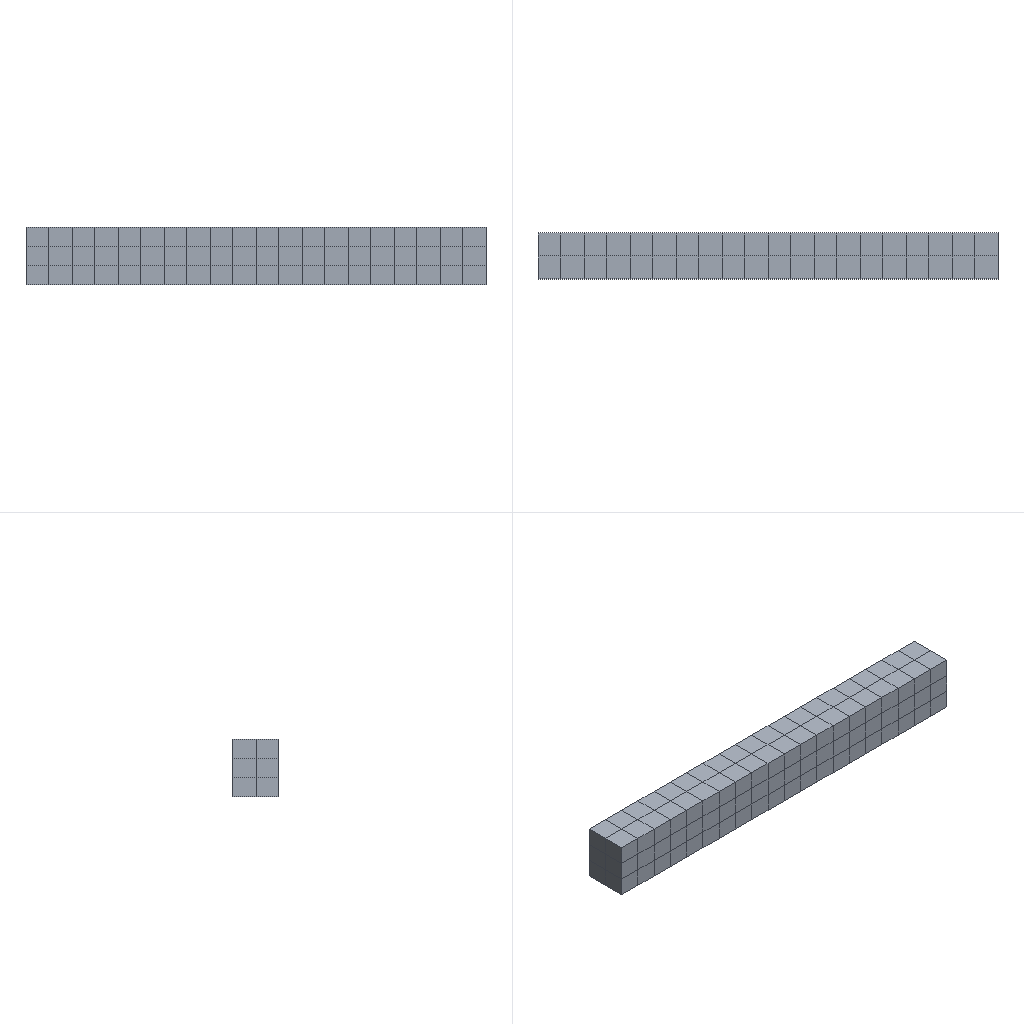Simulation study | abaqus
Set-up summary:
category,name,step,type,value,unit,region
solver,abaqus,,Abaqus/CAE 2024
units,mm-N-s-tonne (MPa),,inferred,E=209000 density=
analysis,loadbeam,,static,time_period=1
mesh,nodes,,,252
mesh,elements,,,120
element_type,C3D8I,,,120
material,Steel,,E,209000
material,Steel,,nu,0.3
section,Steel,,solid section,,,_PickedSet2
load,Pressure,loadbeam,pressure,0.6,,_PickedSurf5
bc,BC-1,initial,fixed,"[dofs=x,y,z n=3]",,_PickedSet4
Abaqus input file, long lists of numbers shortened:
*Heading
** Job name: deck Model name: Model-1
** Generated by: Abaqus/CAE 2024
*Preprint, echo=NO, model=NO, history=NO, contact=NO
**
** PARTS
**
*Part, name=beam
*Node
      1,        -100.,         -10.,          25.
      2,        -100.,           0.,          25.
** (250 more lines like these left out)
*Element, type=C3D8I
  1,  13,  14,  17,  16,   1,   2,   5,   4
  2,  14,  15,  18,  17,   2,   3,   6,   5
** (118 more lines like these left out)
*Nset, nset=_PickedSet2, internal, generate
   1,  252,    1
*Elset, elset=_PickedSet2, internal, generate
   1,  120,    1
** Section: Beamsection
*Solid Section, elset=_PickedSet2, material=Steel
1.,
*End Part
**
**
** ASSEMBLY
**
*Assembly, name=Assembly
**
*Instance, name=beam-1, part=beam
*End Instance
**
*Nset, nset=_PickedSet4, internal, instance=beam-1, generate
  1,  12,   1
*Elset, elset=_PickedSet4, internal, instance=beam-1, generate
 1,  6,  1
*Elset, elset=__PickedSurf5_S5, internal, instance=beam-1
   5,   6,  11,  12,  17,  18,  23,  24,  29,  30,  35,  36,  41,  42,  47,  48
  53,  54,  59,  60,  65,  66,  71,  72,  77,  78,  83,  84,  89,  90,  95,  96
** (1 more lines like these left out)
*Surface, type=ELEMENT, name=_PickedSurf5, internal
__PickedSurf5_S5, S5
*End Assembly
**
** MATERIALS
**
*Material, name=Steel
*Elastic
209000., 0.3
**
** BOUNDARY CONDITIONS
**
** Name: BC-1 Type: Displacement/Rotation
*Boundary
_PickedSet4, 1, 1
_PickedSet4, 2, 2
_PickedSet4, 3, 3
** ----------------------------------------------------------------
**
** STEP: loadbeam
**
*Step, name=loadbeam, nlgeom=NO
Load the top of the
beam
*Static
1., 1., 1e-05, 1.
**
** LOADS
**
** Name: Pressure   Type: Pressure
*Dsload
_PickedSurf5, P, 0.6
**
** OUTPUT REQUESTS
**
*Restart, write, frequency=0
*Print, solve=NO
**
** FIELD OUTPUT: F-Output-1
**
*Output, field, variable=PRESELECT
**
** HISTORY OUTPUT: H-Output-1
**
*Output, history, variable=PRESELECT
*End Step
Results summary:
result,odb.job_status,,,JOB_STATUS_COMPLETED_SUCCESSFULLY,"consistent, unstated (Abaqus has no unit system)"
result,steps[0].procedure,loadbeam,,*STATIC,"consistent, unstated (Abaqus has no unit system)"
result,steps[0].time_period,loadbeam,,1,"consistent, unstated (Abaqus has no unit system)"
result,steps[0].n_frames,loadbeam,,2,"consistent, unstated (Abaqus has no unit system)"
result,steps[0].last_frame.id,loadbeam,,1,"consistent, unstated (Abaqus has no unit system)"
result,steps[0].last_frame.value,loadbeam,,1,"consistent, unstated (Abaqus has no unit system)"
result,steps[0].last_frame.description,loadbeam,,Increment      1: Step Time =    1.000,"consistent, unstated (Abaqus has no unit system)"
result,steps[0].completed,loadbeam,,True,"consistent, unstated (Abaqus has no unit system)"
result,steps[0].max_U_magnitude,loadbeam,,0.4424,"consistent, unstated (Abaqus has no unit system)"
result,steps[0].max_S_mises,loadbeam,,92.677,"consistent, unstated (Abaqus has no unit system)"
result,steps[0].RF_sum[1],loadbeam,,0.0008545,"consistent, unstated (Abaqus has no unit system)"
result,steps[0].RF_sum[2],loadbeam,,0,"consistent, unstated (Abaqus has no unit system)"
result,steps[0].RF_sum[3],loadbeam,,-2400,"consistent, unstated (Abaqus has no unit system)"
result,steps[0].diagnostic.n_increments,loadbeam,,1,"consistent, unstated (Abaqus has no unit system)"